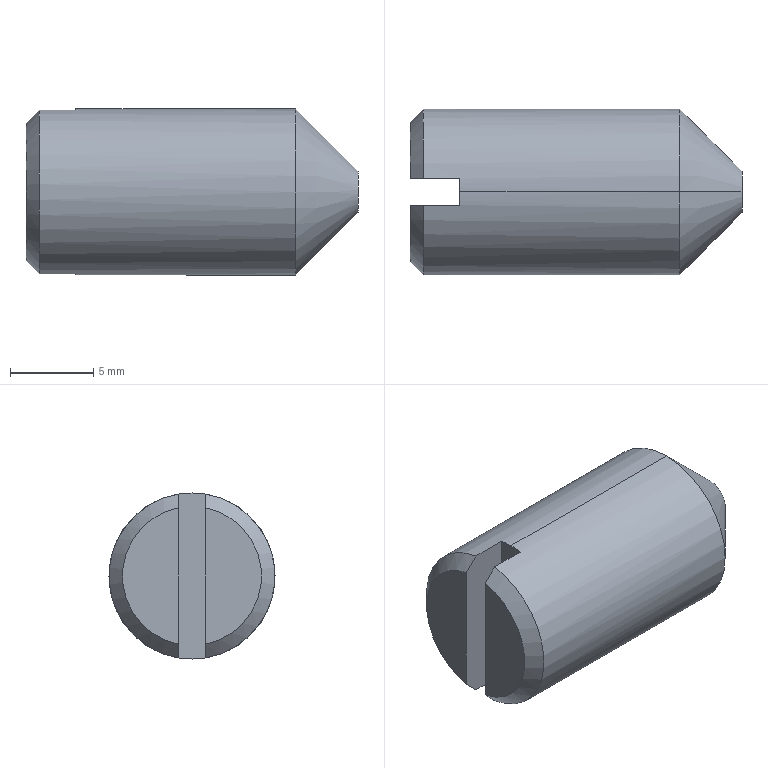Part | SolidWorks | features Cut 1, LPattern 1, RevCut 1, Revolution 1 | 1 solid | 12 faces | box 20 x 10 x 10 mm | volume 1349 mm3 | plane 6 | cone 4 | cylinder 2 | commonest cylinder face diameters 10 x2
STEP:
#1=CARTESIAN_POINT('',(16.25,0.,5.));
#2=VERTEX_POINT('',#1);
#3=CARTESIAN_POINT('',(16.25,0.,-5.));
#4=VERTEX_POINT('',#3);
#5=CARTESIAN_POINT('',(16.25,0.,0.));
#6=DIRECTION('',(-1.,0.,0.));
#7=DIRECTION('',(0.,0.,1.));
#8=AXIS2_PLACEMENT_3D('',#5,#6,#7);
#9=CIRCLE('',#8,5.);
#10=EDGE_CURVE('',#2,#4,#9,.T.);
#11=ORIENTED_EDGE('',*,*,#10,.T.);
#12=CARTESIAN_POINT('',(3.,0.,-5.));
#13=VERTEX_POINT('',#12);
#14=CARTESIAN_POINT('',(-14.774,0.,-5.));
#15=DIRECTION('',(-1.,0.,0.));
#16=VECTOR('',#15,1000.);
#17=LINE('',#14,#16);
#18=EDGE_CURVE('',#4,#13,#17,.T.);
#19=ORIENTED_EDGE('',*,*,#18,.T.);
#20=CARTESIAN_POINT('',(3.,0.8,-4.936));
#21=VERTEX_POINT('',#20);
#22=CARTESIAN_POINT('',(3.,0.,0.));
#23=DIRECTION('',(1.,0.,0.));
#24=DIRECTION('',(0.,0.,-1.));
#25=AXIS2_PLACEMENT_3D('',#22,#23,#24);
#26=CIRCLE('',#25,5.);
#27=EDGE_CURVE('',#13,#21,#26,.T.);
#28=ORIENTED_EDGE('',*,*,#27,.T.);
#29=CARTESIAN_POINT('',(0.812,0.8,-4.936));
#30=VERTEX_POINT('',#29);
#31=CARTESIAN_POINT('',(-14.774,0.8,-4.936));
#32=DIRECTION('',(-1.,0.,0.));
#33=VECTOR('',#32,1000.);
#34=LINE('',#31,#33);
#35=EDGE_CURVE('',#21,#30,#34,.T.);
#36=ORIENTED_EDGE('',*,*,#35,.T.);
#37=CARTESIAN_POINT('',(0.812,0.8,4.936));
#38=VERTEX_POINT('',#37);
#39=CARTESIAN_POINT('',(0.812,0.,0.));
#40=DIRECTION('',(-1.,0.,0.));
#41=DIRECTION('',(0.,0.,1.));
#42=AXIS2_PLACEMENT_3D('',#39,#40,#41);
#43=CIRCLE('',#42,5.);
#44=EDGE_CURVE('',#38,#30,#43,.T.);
#45=ORIENTED_EDGE('',*,*,#44,.F.);
#46=CARTESIAN_POINT('',(3.,0.8,4.936));
#47=VERTEX_POINT('',#46);
#48=CARTESIAN_POINT('',(-14.774,0.8,4.936));
#49=DIRECTION('',(1.,0.,0.));
#50=VECTOR('',#49,1000.);
#51=LINE('',#48,#50);
#52=EDGE_CURVE('',#38,#47,#51,.T.);
#53=ORIENTED_EDGE('',*,*,#52,.T.);
#54=CARTESIAN_POINT('',(3.,0.,5.));
#55=VERTEX_POINT('',#54);
#56=CARTESIAN_POINT('',(3.,0.,0.));
#57=DIRECTION('',(1.,0.,0.));
#58=DIRECTION('',(0.,0.,-1.));
#59=AXIS2_PLACEMENT_3D('',#56,#57,#58);
#60=CIRCLE('',#59,5.);
#61=EDGE_CURVE('',#47,#55,#60,.T.);
#62=ORIENTED_EDGE('',*,*,#61,.T.);
#63=CARTESIAN_POINT('',(-14.774,0.,5.));
#64=DIRECTION('',(-1.,0.,0.));
#65=VECTOR('',#64,1000.);
#66=LINE('',#63,#65);
#67=EDGE_CURVE('',#2,#55,#66,.T.);
#68=ORIENTED_EDGE('',*,*,#67,.F.);
#69=EDGE_LOOP('',(#11,#19,#28,#36,#45,#53,#62,#68));
#70=FACE_OUTER_BOUND('',#69,.T.);
#71=CARTESIAN_POINT('',(-14.774,0.,0.));
#72=DIRECTION('',(-1.,0.,0.));
#73=DIRECTION('',(0.,0.,1.));
#74=AXIS2_PLACEMENT_3D('',#71,#72,#73);
#75=CYLINDRICAL_SURFACE('',#74,5.);
#76=ADVANCED_FACE('',(#70),#75,.T.);
#77=CARTESIAN_POINT('',(20.,0.,1.25));
#78=VERTEX_POINT('',#77);
#79=CARTESIAN_POINT('',(20.,0.,-1.25));
#80=VERTEX_POINT('',#79);
#81=CARTESIAN_POINT('',(20.,0.,0.));
#82=DIRECTION('',(-1.,0.,0.));
#83=DIRECTION('',(0.,0.,1.));
#84=AXIS2_PLACEMENT_3D('',#81,#82,#83);
#85=CIRCLE('',#84,1.25);
#86=EDGE_CURVE('',#78,#80,#85,.T.);
#87=ORIENTED_EDGE('',*,*,#86,.T.);
#88=CARTESIAN_POINT('',(20.,0.,-1.25));
#89=DIRECTION('',(-0.7071,0.,-0.7071));
#90=VECTOR('',#89,1000.);
#91=LINE('',#88,#90);
#92=EDGE_CURVE('',#80,#4,#91,.T.);
#93=ORIENTED_EDGE('',*,*,#92,.T.);
#94=ORIENTED_EDGE('',*,*,#10,.F.);
#95=CARTESIAN_POINT('',(20.,0.,1.25));
#96=DIRECTION('',(-0.7071,0.,0.7071));
#97=VECTOR('',#96,1000.);
#98=LINE('',#95,#97);
#99=EDGE_CURVE('',#78,#2,#98,.T.);
#100=ORIENTED_EDGE('',*,*,#99,.F.);
#101=EDGE_LOOP('',(#87,#93,#94,#100));
#102=FACE_OUTER_BOUND('',#101,.T.);
#103=CARTESIAN_POINT('',(20.,0.,0.));
#104=DIRECTION('',(-1.,0.,0.));
#105=DIRECTION('',(0.,0.,1.));
#106=AXIS2_PLACEMENT_3D('',#103,#104,#105);
#107=CONICAL_SURFACE('',#106,1.25,0.7854);
#108=ADVANCED_FACE('',(#102),#107,.T.);
#109=CARTESIAN_POINT('',(0.,0.8,4.111));
#110=VERTEX_POINT('',#109);
#111=CARTESIAN_POINT('',(0.,0.8,-4.111));
#112=VERTEX_POINT('',#111);
#113=CARTESIAN_POINT('',(0.,0.,0.));
#114=DIRECTION('',(-1.,0.,0.));
#115=DIRECTION('',(0.,0.,1.));
#116=AXIS2_PLACEMENT_3D('',#113,#114,#115);
#117=CIRCLE('',#116,4.188);
#118=EDGE_CURVE('',#110,#112,#117,.T.);
#119=ORIENTED_EDGE('',*,*,#118,.T.);
#120=CARTESIAN_POINT('',(0.,0.8,-5.));
#121=DIRECTION('',(0.,0.,1.));
#122=VECTOR('',#121,1000.);
#123=LINE('',#120,#122);
#124=EDGE_CURVE('',#112,#110,#123,.T.);
#125=ORIENTED_EDGE('',*,*,#124,.T.);
#126=EDGE_LOOP('',(#119,#125));
#127=FACE_OUTER_BOUND('',#126,.T.);
#128=CARTESIAN_POINT('',(0.,4.188,0.));
#129=DIRECTION('',(1.,0.,0.));
#130=DIRECTION('',(0.,0.,-1.));
#131=AXIS2_PLACEMENT_3D('',#128,#129,#130);
#132=PLANE('',#131);
#133=ADVANCED_FACE('',(#127),#132,.F.);
#134=ORIENTED_EDGE('',*,*,#44,.T.);
#135=CARTESIAN_POINT('',(0.812,0.8,-4.936));
#136=CARTESIAN_POINT('',(0.541,0.8,-4.661));
#137=CARTESIAN_POINT('',(0.2702,0.8,-4.386));
#138=CARTESIAN_POINT('',(0.,0.8,-4.111));
#139=B_SPLINE_CURVE_WITH_KNOTS('',3,(#135,#136,#137,#138),.UNSPECIFIED.,.F.,.F.,(4,4),(0.008538,0.009696),.UNSPECIFIED.);
#140=EDGE_CURVE('',#30,#112,#139,.T.);
#141=ORIENTED_EDGE('',*,*,#140,.T.);
#142=ORIENTED_EDGE('',*,*,#118,.F.);
#143=CARTESIAN_POINT('',(0.,0.8,4.111));
#144=CARTESIAN_POINT('',(0.2702,0.8,4.386));
#145=CARTESIAN_POINT('',(0.541,0.8,4.661));
#146=CARTESIAN_POINT('',(0.812,0.8,4.936));
#147=B_SPLINE_CURVE_WITH_KNOTS('',3,(#143,#144,#145,#146),.UNSPECIFIED.,.F.,.F.,(4,4),(0.0205,0.02167),.UNSPECIFIED.);
#148=EDGE_CURVE('',#110,#38,#147,.T.);
#149=ORIENTED_EDGE('',*,*,#148,.T.);
#150=EDGE_LOOP('',(#134,#141,#142,#149));
#151=FACE_OUTER_BOUND('',#150,.T.);
#152=CARTESIAN_POINT('',(0.812,0.,0.));
#153=DIRECTION('',(1.,0.,0.));
#154=DIRECTION('',(0.,0.,-1.));
#155=AXIS2_PLACEMENT_3D('',#152,#153,#154);
#156=CONICAL_SURFACE('',#155,5.,0.7854);
#157=ADVANCED_FACE('',(#151),#156,.T.);
#158=CARTESIAN_POINT('',(0.,-0.8,-4.111));
#159=VERTEX_POINT('',#158);
#160=CARTESIAN_POINT('',(0.,-0.8,4.111));
#161=VERTEX_POINT('',#160);
#162=CARTESIAN_POINT('',(0.,0.,0.));
#163=DIRECTION('',(-1.,0.,0.));
#164=DIRECTION('',(0.,0.,1.));
#165=AXIS2_PLACEMENT_3D('',#162,#163,#164);
#166=CIRCLE('',#165,4.188);
#167=EDGE_CURVE('',#159,#161,#166,.T.);
#168=ORIENTED_EDGE('',*,*,#167,.T.);
#169=CARTESIAN_POINT('',(0.,-0.8,-5.));
#170=DIRECTION('',(0.,0.,1.));
#171=VECTOR('',#170,1000.);
#172=LINE('',#169,#171);
#173=EDGE_CURVE('',#159,#161,#172,.T.);
#174=ORIENTED_EDGE('',*,*,#173,.F.);
#175=EDGE_LOOP('',(#168,#174));
#176=FACE_OUTER_BOUND('',#175,.T.);
#177=CARTESIAN_POINT('',(0.,4.188,0.));
#178=DIRECTION('',(1.,0.,0.));
#179=DIRECTION('',(0.,0.,-1.));
#180=AXIS2_PLACEMENT_3D('',#177,#178,#179);
#181=PLANE('',#180);
#182=ADVANCED_FACE('',(#176),#181,.F.);
#183=ORIENTED_EDGE('',*,*,#86,.F.);
#184=CARTESIAN_POINT('',(20.,0.,0.));
#185=DIRECTION('',(-1.,0.,0.));
#186=DIRECTION('',(0.,0.,1.));
#187=AXIS2_PLACEMENT_3D('',#184,#185,#186);
#188=CIRCLE('',#187,1.25);
#189=EDGE_CURVE('',#80,#78,#188,.T.);
#190=ORIENTED_EDGE('',*,*,#189,.F.);
#191=EDGE_LOOP('',(#183,#190));
#192=FACE_OUTER_BOUND('',#191,.T.);
#193=CARTESIAN_POINT('',(20.,0.,0.));
#194=DIRECTION('',(-1.,0.,0.));
#195=DIRECTION('',(0.,0.,1.));
#196=AXIS2_PLACEMENT_3D('',#193,#194,#195);
#197=PLANE('',#196);
#198=ADVANCED_FACE('',(#192),#197,.F.);
#199=ORIENTED_EDGE('',*,*,#92,.F.);
#200=ORIENTED_EDGE('',*,*,#189,.T.);
#201=ORIENTED_EDGE('',*,*,#99,.T.);
#202=CARTESIAN_POINT('',(16.25,0.,0.));
#203=DIRECTION('',(-1.,0.,0.));
#204=DIRECTION('',(0.,0.,1.));
#205=AXIS2_PLACEMENT_3D('',#202,#203,#204);
#206=CIRCLE('',#205,5.);
#207=EDGE_CURVE('',#4,#2,#206,.T.);
#208=ORIENTED_EDGE('',*,*,#207,.F.);
#209=EDGE_LOOP('',(#199,#200,#201,#208));
#210=FACE_OUTER_BOUND('',#209,.T.);
#211=CARTESIAN_POINT('',(20.,0.,0.));
#212=DIRECTION('',(-1.,0.,0.));
#213=DIRECTION('',(0.,0.,1.));
#214=AXIS2_PLACEMENT_3D('',#211,#212,#213);
#215=CONICAL_SURFACE('',#214,1.25,0.7854);
#216=ADVANCED_FACE('',(#210),#215,.T.);
#217=ORIENTED_EDGE('',*,*,#18,.F.);
#218=ORIENTED_EDGE('',*,*,#207,.T.);
#219=ORIENTED_EDGE('',*,*,#67,.T.);
#220=CARTESIAN_POINT('',(3.,-0.8,4.936));
#221=VERTEX_POINT('',#220);
#222=CARTESIAN_POINT('',(3.,0.,0.));
#223=DIRECTION('',(1.,0.,0.));
#224=DIRECTION('',(0.,0.,-1.));
#225=AXIS2_PLACEMENT_3D('',#222,#223,#224);
#226=CIRCLE('',#225,5.);
#227=EDGE_CURVE('',#55,#221,#226,.T.);
#228=ORIENTED_EDGE('',*,*,#227,.T.);
#229=CARTESIAN_POINT('',(0.812,-0.8,4.936));
#230=VERTEX_POINT('',#229);
#231=CARTESIAN_POINT('',(-14.774,-0.8,4.936));
#232=DIRECTION('',(-1.,0.,0.));
#233=VECTOR('',#232,1000.);
#234=LINE('',#231,#233);
#235=EDGE_CURVE('',#221,#230,#234,.T.);
#236=ORIENTED_EDGE('',*,*,#235,.T.);
#237=CARTESIAN_POINT('',(0.812,-0.8,-4.936));
#238=VERTEX_POINT('',#237);
#239=CARTESIAN_POINT('',(0.812,0.,0.));
#240=DIRECTION('',(-1.,0.,0.));
#241=DIRECTION('',(0.,0.,1.));
#242=AXIS2_PLACEMENT_3D('',#239,#240,#241);
#243=CIRCLE('',#242,5.);
#244=EDGE_CURVE('',#238,#230,#243,.T.);
#245=ORIENTED_EDGE('',*,*,#244,.F.);
#246=CARTESIAN_POINT('',(3.,-0.8,-4.936));
#247=VERTEX_POINT('',#246);
#248=CARTESIAN_POINT('',(-14.774,-0.8,-4.936));
#249=DIRECTION('',(1.,0.,0.));
#250=VECTOR('',#249,1000.);
#251=LINE('',#248,#250);
#252=EDGE_CURVE('',#238,#247,#251,.T.);
#253=ORIENTED_EDGE('',*,*,#252,.T.);
#254=CARTESIAN_POINT('',(3.,0.,0.));
#255=DIRECTION('',(1.,0.,0.));
#256=DIRECTION('',(0.,0.,-1.));
#257=AXIS2_PLACEMENT_3D('',#254,#255,#256);
#258=CIRCLE('',#257,5.);
#259=EDGE_CURVE('',#247,#13,#258,.T.);
#260=ORIENTED_EDGE('',*,*,#259,.T.);
#261=EDGE_LOOP('',(#217,#218,#219,#228,#236,#245,#253,#260));
#262=FACE_OUTER_BOUND('',#261,.T.);
#263=CARTESIAN_POINT('',(-14.774,0.,0.));
#264=DIRECTION('',(-1.,0.,0.));
#265=DIRECTION('',(0.,0.,1.));
#266=AXIS2_PLACEMENT_3D('',#263,#264,#265);
#267=CYLINDRICAL_SURFACE('',#266,5.);
#268=ADVANCED_FACE('',(#262),#267,.T.);
#269=ORIENTED_EDGE('',*,*,#244,.T.);
#270=CARTESIAN_POINT('',(0.812,-0.8,4.936));
#271=CARTESIAN_POINT('',(0.541,-0.8,4.661));
#272=CARTESIAN_POINT('',(0.2702,-0.8,4.386));
#273=CARTESIAN_POINT('',(0.,-0.8,4.111));
#274=B_SPLINE_CURVE_WITH_KNOTS('',3,(#270,#271,#272,#273),.UNSPECIFIED.,.F.,.F.,(4,4),(0.008538,0.009696),.UNSPECIFIED.);
#275=EDGE_CURVE('',#230,#161,#274,.T.);
#276=ORIENTED_EDGE('',*,*,#275,.T.);
#277=ORIENTED_EDGE('',*,*,#167,.F.);
#278=CARTESIAN_POINT('',(0.,-0.8,-4.111));
#279=CARTESIAN_POINT('',(0.2702,-0.8,-4.386));
#280=CARTESIAN_POINT('',(0.541,-0.8,-4.661));
#281=CARTESIAN_POINT('',(0.812,-0.8,-4.936));
#282=B_SPLINE_CURVE_WITH_KNOTS('',3,(#278,#279,#280,#281),.UNSPECIFIED.,.F.,.F.,(4,4),(0.0205,0.02167),.UNSPECIFIED.);
#283=EDGE_CURVE('',#159,#238,#282,.T.);
#284=ORIENTED_EDGE('',*,*,#283,.T.);
#285=EDGE_LOOP('',(#269,#276,#277,#284));
#286=FACE_OUTER_BOUND('',#285,.T.);
#287=CARTESIAN_POINT('',(0.812,0.,0.));
#288=DIRECTION('',(1.,0.,0.));
#289=DIRECTION('',(0.,0.,-1.));
#290=AXIS2_PLACEMENT_3D('',#287,#288,#289);
#291=CONICAL_SURFACE('',#290,5.,0.7854);
#292=ADVANCED_FACE('',(#286),#291,.T.);
#293=CARTESIAN_POINT('',(3.,0.8,-5.));
#294=DIRECTION('',(0.,0.,1.));
#295=VECTOR('',#294,1000.);
#296=LINE('',#293,#295);
#297=EDGE_CURVE('',#21,#47,#296,.T.);
#298=ORIENTED_EDGE('',*,*,#297,.F.);
#299=ORIENTED_EDGE('',*,*,#27,.F.);
#300=ORIENTED_EDGE('',*,*,#259,.F.);
#301=CARTESIAN_POINT('',(3.,-0.8,-5.));
#302=DIRECTION('',(0.,0.,1.));
#303=VECTOR('',#302,1000.);
#304=LINE('',#301,#303);
#305=EDGE_CURVE('',#247,#221,#304,.T.);
#306=ORIENTED_EDGE('',*,*,#305,.T.);
#307=ORIENTED_EDGE('',*,*,#227,.F.);
#308=ORIENTED_EDGE('',*,*,#61,.F.);
#309=EDGE_LOOP('',(#298,#299,#300,#306,#307,#308));
#310=FACE_OUTER_BOUND('',#309,.T.);
#311=CARTESIAN_POINT('',(3.,0.8,-5.));
#312=DIRECTION('',(1.,0.,0.));
#313=DIRECTION('',(0.,0.,-1.));
#314=AXIS2_PLACEMENT_3D('',#311,#312,#313);
#315=PLANE('',#314);
#316=ADVANCED_FACE('',(#310),#315,.F.);
#317=ORIENTED_EDGE('',*,*,#297,.T.);
#318=ORIENTED_EDGE('',*,*,#52,.F.);
#319=ORIENTED_EDGE('',*,*,#148,.F.);
#320=ORIENTED_EDGE('',*,*,#124,.F.);
#321=ORIENTED_EDGE('',*,*,#140,.F.);
#322=ORIENTED_EDGE('',*,*,#35,.F.);
#323=EDGE_LOOP('',(#317,#318,#319,#320,#321,#322));
#324=FACE_OUTER_BOUND('',#323,.T.);
#325=CARTESIAN_POINT('',(0.,0.8,-5.));
#326=DIRECTION('',(0.,1.,0.));
#327=DIRECTION('',(0.,0.,1.));
#328=AXIS2_PLACEMENT_3D('',#325,#326,#327);
#329=PLANE('',#328);
#330=ADVANCED_FACE('',(#324),#329,.F.);
#331=ORIENTED_EDGE('',*,*,#305,.F.);
#332=ORIENTED_EDGE('',*,*,#252,.F.);
#333=ORIENTED_EDGE('',*,*,#283,.F.);
#334=ORIENTED_EDGE('',*,*,#173,.T.);
#335=ORIENTED_EDGE('',*,*,#275,.F.);
#336=ORIENTED_EDGE('',*,*,#235,.F.);
#337=EDGE_LOOP('',(#331,#332,#333,#334,#335,#336));
#338=FACE_OUTER_BOUND('',#337,.T.);
#339=CARTESIAN_POINT('',(0.,-0.8,-5.));
#340=DIRECTION('',(0.,-1.,0.));
#341=DIRECTION('',(0.,0.,-1.));
#342=AXIS2_PLACEMENT_3D('',#339,#340,#341);
#343=PLANE('',#342);
#344=ADVANCED_FACE('',(#338),#343,.F.);
#345=CLOSED_SHELL('',(#76,#108,#133,#157,#182,#198,#216,#268,#292,#316,#330,#344));
#346=MANIFOLD_SOLID_BREP('',#345);
#347=CARTESIAN_POINT('',(0.,0.,0.));
#348=DIRECTION('',(0.,0.,1.));
#349=DIRECTION('',(1.,0.,0.));
#350=AXIS2_PLACEMENT_3D('',#347,#348,#349);
#351=(LENGTH_UNIT()NAMED_UNIT(*)SI_UNIT(.MILLI.,.METRE.));
#352=UNCERTAINTY_MEASURE_WITH_UNIT(LENGTH_MEASURE(0.00001),#351,'','');
#353=(NAMED_UNIT(*)PLANE_ANGLE_UNIT()SI_UNIT($,.RADIAN.));
#354=(NAMED_UNIT(*)SI_UNIT($,.STERADIAN.)SOLID_ANGLE_UNIT());
#355=(GEOMETRIC_REPRESENTATION_CONTEXT(3)GLOBAL_UNCERTAINTY_ASSIGNED_CONTEXT((#352))GLOBAL_UNIT_ASSIGNED_CONTEXT((#351,#353,#354))REPRESENTATION_CONTEXT('',''));
#356=ADVANCED_BREP_SHAPE_REPRESENTATION('',(#346,#350),#355);